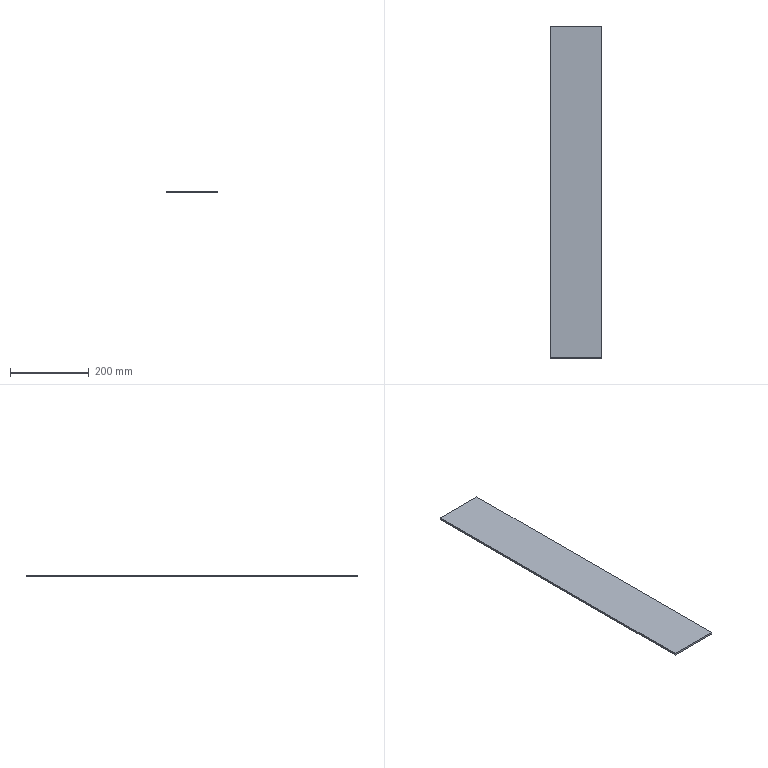Part | SolidWorks | features Extrusion 1, HoleWzd 1 | 1 solid | 6 faces | box 131 x 842 x 5 mm | volume 551510 mm3 | plane 6
STEP:
#1=CARTESIAN_POINT('',(65.5,-421.,0.));
#2=VERTEX_POINT('',#1);
#3=CARTESIAN_POINT('',(65.5,421.,0.));
#4=VERTEX_POINT('',#3);
#5=CARTESIAN_POINT('',(65.5,421.,0.));
#6=DIRECTION('',(0.,1.,0.));
#7=VECTOR('',#6,1000.);
#8=LINE('',#5,#7);
#9=EDGE_CURVE('',#2,#4,#8,.T.);
#10=ORIENTED_EDGE('',*,*,#9,.T.);
#11=CARTESIAN_POINT('',(65.5,421.,5.));
#12=VERTEX_POINT('',#11);
#13=CARTESIAN_POINT('',(65.5,421.,5.));
#14=DIRECTION('',(0.,0.,-1.));
#15=VECTOR('',#14,1000.);
#16=LINE('',#13,#15);
#17=EDGE_CURVE('',#12,#4,#16,.T.);
#18=ORIENTED_EDGE('',*,*,#17,.F.);
#19=CARTESIAN_POINT('',(65.5,-421.,5.));
#20=VERTEX_POINT('',#19);
#21=CARTESIAN_POINT('',(65.5,421.,5.));
#22=DIRECTION('',(0.,1.,0.));
#23=VECTOR('',#22,1000.);
#24=LINE('',#21,#23);
#25=EDGE_CURVE('',#20,#12,#24,.T.);
#26=ORIENTED_EDGE('',*,*,#25,.F.);
#27=CARTESIAN_POINT('',(65.5,-421.,5.));
#28=DIRECTION('',(0.,0.,-1.));
#29=VECTOR('',#28,1000.);
#30=LINE('',#27,#29);
#31=EDGE_CURVE('',#20,#2,#30,.T.);
#32=ORIENTED_EDGE('',*,*,#31,.T.);
#33=EDGE_LOOP('',(#10,#18,#26,#32));
#34=FACE_OUTER_BOUND('',#33,.T.);
#35=CARTESIAN_POINT('',(65.5,421.,5.));
#36=DIRECTION('',(-1.,0.,0.));
#37=DIRECTION('',(0.,-1.,0.));
#38=AXIS2_PLACEMENT_3D('',#35,#36,#37);
#39=PLANE('',#38);
#40=ADVANCED_FACE('',(#34),#39,.F.);
#41=CARTESIAN_POINT('',(-65.5,421.,0.));
#42=VERTEX_POINT('',#41);
#43=CARTESIAN_POINT('',(-65.5,421.,0.));
#44=DIRECTION('',(-1.,0.,0.));
#45=VECTOR('',#44,1000.);
#46=LINE('',#43,#45);
#47=EDGE_CURVE('',#4,#42,#46,.T.);
#48=ORIENTED_EDGE('',*,*,#47,.T.);
#49=CARTESIAN_POINT('',(-65.5,421.,5.));
#50=VERTEX_POINT('',#49);
#51=CARTESIAN_POINT('',(-65.5,421.,5.));
#52=DIRECTION('',(0.,0.,-1.));
#53=VECTOR('',#52,1000.);
#54=LINE('',#51,#53);
#55=EDGE_CURVE('',#50,#42,#54,.T.);
#56=ORIENTED_EDGE('',*,*,#55,.F.);
#57=CARTESIAN_POINT('',(-65.5,421.,5.));
#58=DIRECTION('',(-1.,0.,0.));
#59=VECTOR('',#58,1000.);
#60=LINE('',#57,#59);
#61=EDGE_CURVE('',#12,#50,#60,.T.);
#62=ORIENTED_EDGE('',*,*,#61,.F.);
#63=ORIENTED_EDGE('',*,*,#17,.T.);
#64=EDGE_LOOP('',(#48,#56,#62,#63));
#65=FACE_OUTER_BOUND('',#64,.T.);
#66=CARTESIAN_POINT('',(-65.5,421.,5.));
#67=DIRECTION('',(0.,-1.,0.));
#68=DIRECTION('',(0.,0.,-1.));
#69=AXIS2_PLACEMENT_3D('',#66,#67,#68);
#70=PLANE('',#69);
#71=ADVANCED_FACE('',(#65),#70,.F.);
#72=CARTESIAN_POINT('',(-65.5,-421.,0.));
#73=VERTEX_POINT('',#72);
#74=CARTESIAN_POINT('',(-65.5,421.,0.));
#75=DIRECTION('',(0.,-1.,0.));
#76=VECTOR('',#75,1000.);
#77=LINE('',#74,#76);
#78=EDGE_CURVE('',#42,#73,#77,.T.);
#79=ORIENTED_EDGE('',*,*,#78,.T.);
#80=CARTESIAN_POINT('',(-65.5,-421.,5.));
#81=VERTEX_POINT('',#80);
#82=CARTESIAN_POINT('',(-65.5,-421.,5.));
#83=DIRECTION('',(0.,0.,-1.));
#84=VECTOR('',#83,1000.);
#85=LINE('',#82,#84);
#86=EDGE_CURVE('',#81,#73,#85,.T.);
#87=ORIENTED_EDGE('',*,*,#86,.F.);
#88=CARTESIAN_POINT('',(-65.5,421.,5.));
#89=DIRECTION('',(0.,-1.,0.));
#90=VECTOR('',#89,1000.);
#91=LINE('',#88,#90);
#92=EDGE_CURVE('',#50,#81,#91,.T.);
#93=ORIENTED_EDGE('',*,*,#92,.F.);
#94=ORIENTED_EDGE('',*,*,#55,.T.);
#95=EDGE_LOOP('',(#79,#87,#93,#94));
#96=FACE_OUTER_BOUND('',#95,.T.);
#97=CARTESIAN_POINT('',(-65.5,421.,5.));
#98=DIRECTION('',(1.,0.,0.));
#99=DIRECTION('',(0.,1.,0.));
#100=AXIS2_PLACEMENT_3D('',#97,#98,#99);
#101=PLANE('',#100);
#102=ADVANCED_FACE('',(#96),#101,.F.);
#103=CARTESIAN_POINT('',(-65.5,-421.,0.));
#104=DIRECTION('',(1.,0.,0.));
#105=VECTOR('',#104,1000.);
#106=LINE('',#103,#105);
#107=EDGE_CURVE('',#73,#2,#106,.T.);
#108=ORIENTED_EDGE('',*,*,#107,.T.);
#109=ORIENTED_EDGE('',*,*,#31,.F.);
#110=CARTESIAN_POINT('',(-65.5,-421.,5.));
#111=DIRECTION('',(1.,0.,0.));
#112=VECTOR('',#111,1000.);
#113=LINE('',#110,#112);
#114=EDGE_CURVE('',#81,#20,#113,.T.);
#115=ORIENTED_EDGE('',*,*,#114,.F.);
#116=ORIENTED_EDGE('',*,*,#86,.T.);
#117=EDGE_LOOP('',(#108,#109,#115,#116));
#118=FACE_OUTER_BOUND('',#117,.T.);
#119=CARTESIAN_POINT('',(-65.5,-421.,5.));
#120=DIRECTION('',(0.,1.,0.));
#121=DIRECTION('',(0.,0.,1.));
#122=AXIS2_PLACEMENT_3D('',#119,#120,#121);
#123=PLANE('',#122);
#124=ADVANCED_FACE('',(#118),#123,.F.);
#125=ORIENTED_EDGE('',*,*,#25,.T.);
#126=ORIENTED_EDGE('',*,*,#61,.T.);
#127=ORIENTED_EDGE('',*,*,#92,.T.);
#128=ORIENTED_EDGE('',*,*,#114,.T.);
#129=EDGE_LOOP('',(#125,#126,#127,#128));
#130=FACE_OUTER_BOUND('',#129,.T.);
#131=CARTESIAN_POINT('',(0.,0.,5.));
#132=DIRECTION('',(0.,0.,1.));
#133=DIRECTION('',(1.,0.,0.));
#134=AXIS2_PLACEMENT_3D('',#131,#132,#133);
#135=PLANE('',#134);
#136=ADVANCED_FACE('',(#130),#135,.T.);
#137=ORIENTED_EDGE('',*,*,#9,.F.);
#138=ORIENTED_EDGE('',*,*,#107,.F.);
#139=ORIENTED_EDGE('',*,*,#78,.F.);
#140=ORIENTED_EDGE('',*,*,#47,.F.);
#141=EDGE_LOOP('',(#137,#138,#139,#140));
#142=FACE_OUTER_BOUND('',#141,.T.);
#143=CARTESIAN_POINT('',(0.,0.,0.));
#144=DIRECTION('',(0.,0.,1.));
#145=DIRECTION('',(1.,0.,0.));
#146=AXIS2_PLACEMENT_3D('',#143,#144,#145);
#147=PLANE('',#146);
#148=ADVANCED_FACE('',(#142),#147,.F.);
#149=CLOSED_SHELL('',(#40,#71,#102,#124,#136,#148));
#150=MANIFOLD_SOLID_BREP('',#149);
#151=CARTESIAN_POINT('',(0.,0.,0.));
#152=DIRECTION('',(0.,0.,1.));
#153=DIRECTION('',(1.,0.,0.));
#154=AXIS2_PLACEMENT_3D('',#151,#152,#153);
#155=(LENGTH_UNIT()NAMED_UNIT(*)SI_UNIT(.MILLI.,.METRE.));
#156=UNCERTAINTY_MEASURE_WITH_UNIT(LENGTH_MEASURE(0.00001),#155,'','');
#157=(NAMED_UNIT(*)PLANE_ANGLE_UNIT()SI_UNIT($,.RADIAN.));
#158=(NAMED_UNIT(*)SI_UNIT($,.STERADIAN.)SOLID_ANGLE_UNIT());
#159=(GEOMETRIC_REPRESENTATION_CONTEXT(3)GLOBAL_UNCERTAINTY_ASSIGNED_CONTEXT((#156))GLOBAL_UNIT_ASSIGNED_CONTEXT((#155,#157,#158))REPRESENTATION_CONTEXT('',''));
#160=ADVANCED_BREP_SHAPE_REPRESENTATION('',(#150,#154),#159);